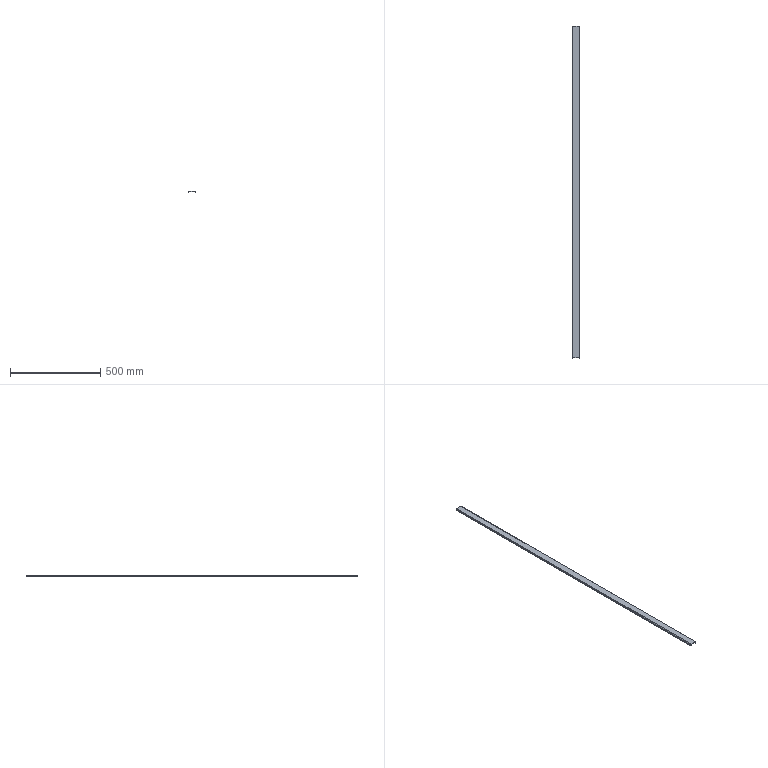Part | SolidWorks | features BaseBody 1 | 1 solid | 22 faces | box 40 x 1838 x 10 mm | volume 245796 mm3 | plane 18 | cylinder 4 | commonest cylinder face diameters 1 x2 6 x2
STEP:
#1=CARTESIAN_POINT('',(-17.5,918.9,-10.));
#2=VERTEX_POINT('',#1);
#3=CARTESIAN_POINT('',(-17.5,-918.9,-10.));
#4=VERTEX_POINT('',#3);
#5=CARTESIAN_POINT('',(-17.5,-918.9,-10.));
#6=DIRECTION('',(0.,-1.,0.));
#7=VECTOR('',#6,1000.);
#8=LINE('',#5,#7);
#9=EDGE_CURVE('',#2,#4,#8,.T.);
#10=ORIENTED_EDGE('',*,*,#9,.T.);
#11=CARTESIAN_POINT('',(-20.,-918.9,-10.));
#12=VERTEX_POINT('',#11);
#13=CARTESIAN_POINT('',(-20.,-918.9,-10.));
#14=DIRECTION('',(1.,0.,0.));
#15=VECTOR('',#14,1000.);
#16=LINE('',#13,#15);
#17=EDGE_CURVE('',#12,#4,#16,.T.);
#18=ORIENTED_EDGE('',*,*,#17,.F.);
#19=CARTESIAN_POINT('',(-20.,918.9,-10.));
#20=VERTEX_POINT('',#19);
#21=CARTESIAN_POINT('',(-20.,0.,-10.));
#22=DIRECTION('',(0.,-1.,0.));
#23=VECTOR('',#22,1000.);
#24=LINE('',#21,#23);
#25=EDGE_CURVE('',#20,#12,#24,.T.);
#26=ORIENTED_EDGE('',*,*,#25,.F.);
#27=CARTESIAN_POINT('',(-20.,918.9,-10.));
#28=DIRECTION('',(1.,0.,0.));
#29=VECTOR('',#28,1000.);
#30=LINE('',#27,#29);
#31=EDGE_CURVE('',#20,#2,#30,.T.);
#32=ORIENTED_EDGE('',*,*,#31,.T.);
#33=EDGE_LOOP('',(#10,#18,#26,#32));
#34=FACE_OUTER_BOUND('',#33,.T.);
#35=CARTESIAN_POINT('',(-20.,-918.9,-10.));
#36=DIRECTION('',(0.,0.,1.));
#37=DIRECTION('',(1.,0.,0.));
#38=AXIS2_PLACEMENT_3D('',#35,#36,#37);
#39=PLANE('',#38);
#40=ADVANCED_FACE('',(#34),#39,.F.);
#41=CARTESIAN_POINT('',(-17.5,918.9,-3.));
#42=VERTEX_POINT('',#41);
#43=CARTESIAN_POINT('',(-17.5,918.9,-10.));
#44=DIRECTION('',(0.,0.,-1.));
#45=VECTOR('',#44,1000.);
#46=LINE('',#43,#45);
#47=EDGE_CURVE('',#42,#2,#46,.T.);
#48=ORIENTED_EDGE('',*,*,#47,.F.);
#49=CARTESIAN_POINT('',(-17.5,-918.9,-3.));
#50=VERTEX_POINT('',#49);
#51=CARTESIAN_POINT('',(-17.5,-918.9,-3.));
#52=DIRECTION('',(0.,1.,0.));
#53=VECTOR('',#52,1000.);
#54=LINE('',#51,#53);
#55=EDGE_CURVE('',#50,#42,#54,.T.);
#56=ORIENTED_EDGE('',*,*,#55,.F.);
#57=CARTESIAN_POINT('',(-17.5,-918.9,-2.5));
#58=DIRECTION('',(0.,0.,1.));
#59=VECTOR('',#58,1000.);
#60=LINE('',#57,#59);
#61=EDGE_CURVE('',#4,#50,#60,.T.);
#62=ORIENTED_EDGE('',*,*,#61,.F.);
#63=ORIENTED_EDGE('',*,*,#9,.F.);
#64=EDGE_LOOP('',(#48,#56,#62,#63));
#65=FACE_OUTER_BOUND('',#64,.T.);
#66=CARTESIAN_POINT('',(-17.5,0.,0.));
#67=DIRECTION('',(1.,0.,0.));
#68=DIRECTION('',(0.,0.,-1.));
#69=AXIS2_PLACEMENT_3D('',#66,#67,#68);
#70=PLANE('',#69);
#71=ADVANCED_FACE('',(#65),#70,.T.);
#72=CARTESIAN_POINT('',(-20.,918.9,-3.));
#73=VERTEX_POINT('',#72);
#74=CARTESIAN_POINT('',(-20.,-918.9,-3.));
#75=VERTEX_POINT('',#74);
#76=CARTESIAN_POINT('',(-20.,-918.9,-3.));
#77=DIRECTION('',(0.,-1.,0.));
#78=VECTOR('',#77,1000.);
#79=LINE('',#76,#78);
#80=EDGE_CURVE('',#73,#75,#79,.T.);
#81=ORIENTED_EDGE('',*,*,#80,.F.);
#82=CARTESIAN_POINT('',(-20.,918.9,0.));
#83=DIRECTION('',(0.,0.,-1.));
#84=VECTOR('',#83,1000.);
#85=LINE('',#82,#84);
#86=EDGE_CURVE('',#73,#20,#85,.T.);
#87=ORIENTED_EDGE('',*,*,#86,.T.);
#88=ORIENTED_EDGE('',*,*,#25,.T.);
#89=CARTESIAN_POINT('',(-20.,-918.9,0.));
#90=DIRECTION('',(0.,0.,1.));
#91=VECTOR('',#90,1000.);
#92=LINE('',#89,#91);
#93=EDGE_CURVE('',#12,#75,#92,.T.);
#94=ORIENTED_EDGE('',*,*,#93,.T.);
#95=EDGE_LOOP('',(#81,#87,#88,#94));
#96=FACE_OUTER_BOUND('',#95,.T.);
#97=CARTESIAN_POINT('',(-20.,0.,0.));
#98=DIRECTION('',(1.,0.,0.));
#99=DIRECTION('',(0.,0.,-1.));
#100=AXIS2_PLACEMENT_3D('',#97,#98,#99);
#101=PLANE('',#100);
#102=ADVANCED_FACE('',(#96),#101,.F.);
#103=CARTESIAN_POINT('',(-20.,-918.9,-3.));
#104=DIRECTION('',(-1.,0.,0.));
#105=VECTOR('',#104,1000.);
#106=LINE('',#103,#105);
#107=EDGE_CURVE('',#50,#75,#106,.T.);
#108=ORIENTED_EDGE('',*,*,#107,.T.);
#109=ORIENTED_EDGE('',*,*,#93,.F.);
#110=ORIENTED_EDGE('',*,*,#17,.T.);
#111=ORIENTED_EDGE('',*,*,#61,.T.);
#112=EDGE_LOOP('',(#108,#109,#110,#111));
#113=FACE_OUTER_BOUND('',#112,.T.);
#114=CARTESIAN_POINT('',(-20.,-918.9,-2.5));
#115=DIRECTION('',(0.,1.,0.));
#116=DIRECTION('',(0.,0.,-1.));
#117=AXIS2_PLACEMENT_3D('',#114,#115,#116);
#118=PLANE('',#117);
#119=ADVANCED_FACE('',(#113),#118,.F.);
#120=CARTESIAN_POINT('',(-17.5,918.9,-3.));
#121=DIRECTION('',(-1.,0.,0.));
#122=VECTOR('',#121,1000.);
#123=LINE('',#120,#122);
#124=EDGE_CURVE('',#42,#73,#123,.T.);
#125=ORIENTED_EDGE('',*,*,#124,.F.);
#126=ORIENTED_EDGE('',*,*,#47,.T.);
#127=ORIENTED_EDGE('',*,*,#31,.F.);
#128=ORIENTED_EDGE('',*,*,#86,.F.);
#129=EDGE_LOOP('',(#125,#126,#127,#128));
#130=FACE_OUTER_BOUND('',#129,.T.);
#131=CARTESIAN_POINT('',(-20.,918.9,-10.));
#132=DIRECTION('',(0.,-1.,0.));
#133=DIRECTION('',(-1.,0.,0.));
#134=AXIS2_PLACEMENT_3D('',#131,#132,#133);
#135=PLANE('',#134);
#136=ADVANCED_FACE('',(#130),#135,.F.);
#137=CARTESIAN_POINT('',(-17.,918.9,-2.5));
#138=VERTEX_POINT('',#137);
#139=CARTESIAN_POINT('',(-17.,-918.9,-2.5));
#140=VERTEX_POINT('',#139);
#141=CARTESIAN_POINT('',(-17.,918.9,-2.5));
#142=DIRECTION('',(0.,-1.,0.));
#143=VECTOR('',#142,1000.);
#144=LINE('',#141,#143);
#145=EDGE_CURVE('',#138,#140,#144,.T.);
#146=ORIENTED_EDGE('',*,*,#145,.T.);
#147=CARTESIAN_POINT('',(-17.,-918.9,-3.));
#148=DIRECTION('',(0.,-1.,0.));
#149=DIRECTION('',(0.,0.,1.));
#150=AXIS2_PLACEMENT_3D('',#147,#148,#149);
#151=CIRCLE('',#150,0.5);
#152=EDGE_CURVE('',#140,#50,#151,.T.);
#153=ORIENTED_EDGE('',*,*,#152,.T.);
#154=ORIENTED_EDGE('',*,*,#55,.T.);
#155=CARTESIAN_POINT('',(-17.,918.9,-3.));
#156=DIRECTION('',(0.,1.,0.));
#157=DIRECTION('',(0.,0.,1.));
#158=AXIS2_PLACEMENT_3D('',#155,#156,#157);
#159=CIRCLE('',#158,0.5);
#160=EDGE_CURVE('',#42,#138,#159,.T.);
#161=ORIENTED_EDGE('',*,*,#160,.T.);
#162=EDGE_LOOP('',(#146,#153,#154,#161));
#163=FACE_OUTER_BOUND('',#162,.T.);
#164=CARTESIAN_POINT('',(-17.,918.9,-3.));
#165=DIRECTION('',(0.,1.,0.));
#166=DIRECTION('',(-1.,0.,0.));
#167=AXIS2_PLACEMENT_3D('',#164,#165,#166);
#168=CYLINDRICAL_SURFACE('',#167,0.5);
#169=ADVANCED_FACE('',(#163),#168,.F.);
#170=CARTESIAN_POINT('',(-17.,918.9,0.));
#171=VERTEX_POINT('',#170);
#172=CARTESIAN_POINT('',(-17.,-918.9,0.));
#173=VERTEX_POINT('',#172);
#174=CARTESIAN_POINT('',(-17.,918.9,0.));
#175=DIRECTION('',(0.,-1.,0.));
#176=VECTOR('',#175,1000.);
#177=LINE('',#174,#176);
#178=EDGE_CURVE('',#171,#173,#177,.T.);
#179=ORIENTED_EDGE('',*,*,#178,.F.);
#180=CARTESIAN_POINT('',(-17.,918.9,-3.));
#181=DIRECTION('',(0.,1.,0.));
#182=DIRECTION('',(0.,0.,1.));
#183=AXIS2_PLACEMENT_3D('',#180,#181,#182);
#184=CIRCLE('',#183,3.);
#185=EDGE_CURVE('',#73,#171,#184,.T.);
#186=ORIENTED_EDGE('',*,*,#185,.F.);
#187=ORIENTED_EDGE('',*,*,#80,.T.);
#188=CARTESIAN_POINT('',(-17.,-918.9,-3.));
#189=DIRECTION('',(0.,-1.,0.));
#190=DIRECTION('',(0.,0.,1.));
#191=AXIS2_PLACEMENT_3D('',#188,#189,#190);
#192=CIRCLE('',#191,3.);
#193=EDGE_CURVE('',#173,#75,#192,.T.);
#194=ORIENTED_EDGE('',*,*,#193,.F.);
#195=EDGE_LOOP('',(#179,#186,#187,#194));
#196=FACE_OUTER_BOUND('',#195,.T.);
#197=CARTESIAN_POINT('',(-17.,918.9,-3.));
#198=DIRECTION('',(0.,1.,0.));
#199=DIRECTION('',(-1.,0.,0.));
#200=AXIS2_PLACEMENT_3D('',#197,#198,#199);
#201=CYLINDRICAL_SURFACE('',#200,3.);
#202=ADVANCED_FACE('',(#196),#201,.T.);
#203=ORIENTED_EDGE('',*,*,#160,.F.);
#204=ORIENTED_EDGE('',*,*,#124,.T.);
#205=ORIENTED_EDGE('',*,*,#185,.T.);
#206=CARTESIAN_POINT('',(-17.,918.9,-2.5));
#207=DIRECTION('',(0.,0.,1.));
#208=VECTOR('',#207,1000.);
#209=LINE('',#206,#208);
#210=EDGE_CURVE('',#138,#171,#209,.T.);
#211=ORIENTED_EDGE('',*,*,#210,.F.);
#212=EDGE_LOOP('',(#203,#204,#205,#211));
#213=FACE_OUTER_BOUND('',#212,.T.);
#214=CARTESIAN_POINT('',(-17.,918.9,-3.));
#215=DIRECTION('',(0.,-1.,0.));
#216=DIRECTION('',(0.,0.,-1.));
#217=AXIS2_PLACEMENT_3D('',#214,#215,#216);
#218=PLANE('',#217);
#219=ADVANCED_FACE('',(#213),#218,.F.);
#220=ORIENTED_EDGE('',*,*,#107,.F.);
#221=ORIENTED_EDGE('',*,*,#152,.F.);
#222=CARTESIAN_POINT('',(-17.,-918.9,-2.5));
#223=DIRECTION('',(0.,0.,1.));
#224=VECTOR('',#223,1000.);
#225=LINE('',#222,#224);
#226=EDGE_CURVE('',#140,#173,#225,.T.);
#227=ORIENTED_EDGE('',*,*,#226,.T.);
#228=ORIENTED_EDGE('',*,*,#193,.T.);
#229=EDGE_LOOP('',(#220,#221,#227,#228));
#230=FACE_OUTER_BOUND('',#229,.T.);
#231=CARTESIAN_POINT('',(-17.,-918.9,-3.));
#232=DIRECTION('',(0.,-1.,0.));
#233=DIRECTION('',(0.,0.,-1.));
#234=AXIS2_PLACEMENT_3D('',#231,#232,#233);
#235=PLANE('',#234);
#236=ADVANCED_FACE('',(#230),#235,.T.);
#237=CARTESIAN_POINT('',(17.5,-918.9,-10.));
#238=VERTEX_POINT('',#237);
#239=CARTESIAN_POINT('',(17.5,918.9,-10.));
#240=VERTEX_POINT('',#239);
#241=CARTESIAN_POINT('',(17.5,918.9,-10.));
#242=DIRECTION('',(0.,1.,0.));
#243=VECTOR('',#242,1000.);
#244=LINE('',#241,#243);
#245=EDGE_CURVE('',#238,#240,#244,.T.);
#246=ORIENTED_EDGE('',*,*,#245,.T.);
#247=CARTESIAN_POINT('',(20.,918.9,-10.));
#248=VERTEX_POINT('',#247);
#249=CARTESIAN_POINT('',(20.,918.9,-10.));
#250=DIRECTION('',(-1.,0.,0.));
#251=VECTOR('',#250,1000.);
#252=LINE('',#249,#251);
#253=EDGE_CURVE('',#248,#240,#252,.T.);
#254=ORIENTED_EDGE('',*,*,#253,.F.);
#255=CARTESIAN_POINT('',(20.,-918.9,-10.));
#256=VERTEX_POINT('',#255);
#257=CARTESIAN_POINT('',(20.,0.,-10.));
#258=DIRECTION('',(0.,1.,0.));
#259=VECTOR('',#258,1000.);
#260=LINE('',#257,#259);
#261=EDGE_CURVE('',#256,#248,#260,.T.);
#262=ORIENTED_EDGE('',*,*,#261,.F.);
#263=CARTESIAN_POINT('',(20.,-918.9,-10.));
#264=DIRECTION('',(-1.,0.,0.));
#265=VECTOR('',#264,1000.);
#266=LINE('',#263,#265);
#267=EDGE_CURVE('',#256,#238,#266,.T.);
#268=ORIENTED_EDGE('',*,*,#267,.T.);
#269=EDGE_LOOP('',(#246,#254,#262,#268));
#270=FACE_OUTER_BOUND('',#269,.T.);
#271=CARTESIAN_POINT('',(20.,918.9,-10.));
#272=DIRECTION('',(0.,0.,1.));
#273=DIRECTION('',(1.,0.,0.));
#274=AXIS2_PLACEMENT_3D('',#271,#272,#273);
#275=PLANE('',#274);
#276=ADVANCED_FACE('',(#270),#275,.F.);
#277=CARTESIAN_POINT('',(17.5,-918.9,-3.));
#278=VERTEX_POINT('',#277);
#279=CARTESIAN_POINT('',(17.5,-918.9,-10.));
#280=DIRECTION('',(0.,0.,-1.));
#281=VECTOR('',#280,1000.);
#282=LINE('',#279,#281);
#283=EDGE_CURVE('',#278,#238,#282,.T.);
#284=ORIENTED_EDGE('',*,*,#283,.F.);
#285=CARTESIAN_POINT('',(17.5,918.9,-3.));
#286=VERTEX_POINT('',#285);
#287=CARTESIAN_POINT('',(17.5,918.9,-3.));
#288=DIRECTION('',(0.,-1.,0.));
#289=VECTOR('',#288,1000.);
#290=LINE('',#287,#289);
#291=EDGE_CURVE('',#286,#278,#290,.T.);
#292=ORIENTED_EDGE('',*,*,#291,.F.);
#293=CARTESIAN_POINT('',(17.5,918.9,-2.5));
#294=DIRECTION('',(0.,0.,1.));
#295=VECTOR('',#294,1000.);
#296=LINE('',#293,#295);
#297=EDGE_CURVE('',#240,#286,#296,.T.);
#298=ORIENTED_EDGE('',*,*,#297,.F.);
#299=ORIENTED_EDGE('',*,*,#245,.F.);
#300=EDGE_LOOP('',(#284,#292,#298,#299));
#301=FACE_OUTER_BOUND('',#300,.T.);
#302=CARTESIAN_POINT('',(17.5,0.,0.));
#303=DIRECTION('',(-1.,0.,0.));
#304=DIRECTION('',(0.,0.,1.));
#305=AXIS2_PLACEMENT_3D('',#302,#303,#304);
#306=PLANE('',#305);
#307=ADVANCED_FACE('',(#301),#306,.T.);
#308=CARTESIAN_POINT('',(20.,-918.9,-3.));
#309=VERTEX_POINT('',#308);
#310=CARTESIAN_POINT('',(20.,918.9,-3.));
#311=VERTEX_POINT('',#310);
#312=CARTESIAN_POINT('',(20.,918.9,-3.));
#313=DIRECTION('',(0.,1.,0.));
#314=VECTOR('',#313,1000.);
#315=LINE('',#312,#314);
#316=EDGE_CURVE('',#309,#311,#315,.T.);
#317=ORIENTED_EDGE('',*,*,#316,.F.);
#318=CARTESIAN_POINT('',(20.,-918.9,0.));
#319=DIRECTION('',(0.,0.,-1.));
#320=VECTOR('',#319,1000.);
#321=LINE('',#318,#320);
#322=EDGE_CURVE('',#309,#256,#321,.T.);
#323=ORIENTED_EDGE('',*,*,#322,.T.);
#324=ORIENTED_EDGE('',*,*,#261,.T.);
#325=CARTESIAN_POINT('',(20.,918.9,0.));
#326=DIRECTION('',(0.,0.,1.));
#327=VECTOR('',#326,1000.);
#328=LINE('',#325,#327);
#329=EDGE_CURVE('',#248,#311,#328,.T.);
#330=ORIENTED_EDGE('',*,*,#329,.T.);
#331=EDGE_LOOP('',(#317,#323,#324,#330));
#332=FACE_OUTER_BOUND('',#331,.T.);
#333=CARTESIAN_POINT('',(20.,0.,0.));
#334=DIRECTION('',(-1.,0.,0.));
#335=DIRECTION('',(0.,0.,1.));
#336=AXIS2_PLACEMENT_3D('',#333,#334,#335);
#337=PLANE('',#336);
#338=ADVANCED_FACE('',(#332),#337,.F.);
#339=CARTESIAN_POINT('',(20.,918.9,-3.));
#340=DIRECTION('',(1.,0.,0.));
#341=VECTOR('',#340,1000.);
#342=LINE('',#339,#341);
#343=EDGE_CURVE('',#286,#311,#342,.T.);
#344=ORIENTED_EDGE('',*,*,#343,.T.);
#345=ORIENTED_EDGE('',*,*,#329,.F.);
#346=ORIENTED_EDGE('',*,*,#253,.T.);
#347=ORIENTED_EDGE('',*,*,#297,.T.);
#348=EDGE_LOOP('',(#344,#345,#346,#347));
#349=FACE_OUTER_BOUND('',#348,.T.);
#350=CARTESIAN_POINT('',(20.,918.9,-2.5));
#351=DIRECTION('',(0.,-1.,0.));
#352=DIRECTION('',(-1.,0.,0.));
#353=AXIS2_PLACEMENT_3D('',#350,#351,#352);
#354=PLANE('',#353);
#355=ADVANCED_FACE('',(#349),#354,.F.);
#356=CARTESIAN_POINT('',(17.5,-918.9,-3.));
#357=DIRECTION('',(1.,0.,0.));
#358=VECTOR('',#357,1000.);
#359=LINE('',#356,#358);
#360=EDGE_CURVE('',#278,#309,#359,.T.);
#361=ORIENTED_EDGE('',*,*,#360,.F.);
#362=ORIENTED_EDGE('',*,*,#283,.T.);
#363=ORIENTED_EDGE('',*,*,#267,.F.);
#364=ORIENTED_EDGE('',*,*,#322,.F.);
#365=EDGE_LOOP('',(#361,#362,#363,#364));
#366=FACE_OUTER_BOUND('',#365,.T.);
#367=CARTESIAN_POINT('',(20.,-918.9,-10.));
#368=DIRECTION('',(0.,1.,0.));
#369=DIRECTION('',(0.,0.,-1.));
#370=AXIS2_PLACEMENT_3D('',#367,#368,#369);
#371=PLANE('',#370);
#372=ADVANCED_FACE('',(#366),#371,.F.);
#373=CARTESIAN_POINT('',(17.,-918.9,-2.5));
#374=VERTEX_POINT('',#373);
#375=CARTESIAN_POINT('',(17.,918.9,-2.5));
#376=VERTEX_POINT('',#375);
#377=CARTESIAN_POINT('',(17.,-918.9,-2.5));
#378=DIRECTION('',(0.,1.,0.));
#379=VECTOR('',#378,1000.);
#380=LINE('',#377,#379);
#381=EDGE_CURVE('',#374,#376,#380,.T.);
#382=ORIENTED_EDGE('',*,*,#381,.T.);
#383=CARTESIAN_POINT('',(17.,918.9,-3.));
#384=DIRECTION('',(0.,1.,0.));
#385=DIRECTION('',(0.,0.,-1.));
#386=AXIS2_PLACEMENT_3D('',#383,#384,#385);
#387=CIRCLE('',#386,0.5);
#388=EDGE_CURVE('',#376,#286,#387,.T.);
#389=ORIENTED_EDGE('',*,*,#388,.T.);
#390=ORIENTED_EDGE('',*,*,#291,.T.);
#391=CARTESIAN_POINT('',(17.,-918.9,-3.));
#392=DIRECTION('',(0.,-1.,0.));
#393=DIRECTION('',(0.,0.,-1.));
#394=AXIS2_PLACEMENT_3D('',#391,#392,#393);
#395=CIRCLE('',#394,0.5);
#396=EDGE_CURVE('',#278,#374,#395,.T.);
#397=ORIENTED_EDGE('',*,*,#396,.T.);
#398=EDGE_LOOP('',(#382,#389,#390,#397));
#399=FACE_OUTER_BOUND('',#398,.T.);
#400=CARTESIAN_POINT('',(17.,-918.9,-3.));
#401=DIRECTION('',(0.,-1.,0.));
#402=DIRECTION('',(1.,0.,0.));
#403=AXIS2_PLACEMENT_3D('',#400,#401,#402);
#404=CYLINDRICAL_SURFACE('',#403,0.5);
#405=ADVANCED_FACE('',(#399),#404,.F.);
#406=CARTESIAN_POINT('',(17.,-918.9,0.));
#407=VERTEX_POINT('',#406);
#408=CARTESIAN_POINT('',(17.,918.9,0.));
#409=VERTEX_POINT('',#408);
#410=CARTESIAN_POINT('',(17.,-918.9,0.));
#411=DIRECTION('',(0.,1.,0.));
#412=VECTOR('',#411,1000.);
#413=LINE('',#410,#412);
#414=EDGE_CURVE('',#407,#409,#413,.T.);
#415=ORIENTED_EDGE('',*,*,#414,.F.);
#416=CARTESIAN_POINT('',(17.,-918.9,-3.));
#417=DIRECTION('',(0.,-1.,0.));
#418=DIRECTION('',(0.,0.,-1.));
#419=AXIS2_PLACEMENT_3D('',#416,#417,#418);
#420=CIRCLE('',#419,3.);
#421=EDGE_CURVE('',#309,#407,#420,.T.);
#422=ORIENTED_EDGE('',*,*,#421,.F.);
#423=ORIENTED_EDGE('',*,*,#316,.T.);
#424=CARTESIAN_POINT('',(17.,918.9,-3.));
#425=DIRECTION('',(0.,1.,0.));
#426=DIRECTION('',(0.,0.,-1.));
#427=AXIS2_PLACEMENT_3D('',#424,#425,#426);
#428=CIRCLE('',#427,3.);
#429=EDGE_CURVE('',#409,#311,#428,.T.);
#430=ORIENTED_EDGE('',*,*,#429,.F.);
#431=EDGE_LOOP('',(#415,#422,#423,#430));
#432=FACE_OUTER_BOUND('',#431,.T.);
#433=CARTESIAN_POINT('',(17.,-918.9,-3.));
#434=DIRECTION('',(0.,-1.,0.));
#435=DIRECTION('',(1.,0.,0.));
#436=AXIS2_PLACEMENT_3D('',#433,#434,#435);
#437=CYLINDRICAL_SURFACE('',#436,3.);
#438=ADVANCED_FACE('',(#432),#437,.T.);
#439=ORIENTED_EDGE('',*,*,#396,.F.);
#440=ORIENTED_EDGE('',*,*,#360,.T.);
#441=ORIENTED_EDGE('',*,*,#421,.T.);
#442=CARTESIAN_POINT('',(17.,-918.9,-2.5));
#443=DIRECTION('',(0.,0.,1.));
#444=VECTOR('',#443,1000.);
#445=LINE('',#442,#444);
#446=EDGE_CURVE('',#374,#407,#445,.T.);
#447=ORIENTED_EDGE('',*,*,#446,.F.);
#448=EDGE_LOOP('',(#439,#440,#441,#447));
#449=FACE_OUTER_BOUND('',#448,.T.);
#450=CARTESIAN_POINT('',(17.,-918.9,-3.));
#451=DIRECTION('',(0.,1.,0.));
#452=DIRECTION('',(1.,0.,0.));
#453=AXIS2_PLACEMENT_3D('',#450,#451,#452);
#454=PLANE('',#453);
#455=ADVANCED_FACE('',(#449),#454,.F.);
#456=ORIENTED_EDGE('',*,*,#343,.F.);
#457=ORIENTED_EDGE('',*,*,#388,.F.);
#458=CARTESIAN_POINT('',(17.,918.9,-2.5));
#459=DIRECTION('',(0.,0.,1.));
#460=VECTOR('',#459,1000.);
#461=LINE('',#458,#460);
#462=EDGE_CURVE('',#376,#409,#461,.T.);
#463=ORIENTED_EDGE('',*,*,#462,.T.);
#464=ORIENTED_EDGE('',*,*,#429,.T.);
#465=EDGE_LOOP('',(#456,#457,#463,#464));
#466=FACE_OUTER_BOUND('',#465,.T.);
#467=CARTESIAN_POINT('',(17.,918.9,-3.));
#468=DIRECTION('',(0.,1.,0.));
#469=DIRECTION('',(1.,0.,0.));
#470=AXIS2_PLACEMENT_3D('',#467,#468,#469);
#471=PLANE('',#470);
#472=ADVANCED_FACE('',(#466),#471,.T.);
#473=ORIENTED_EDGE('',*,*,#226,.F.);
#474=CARTESIAN_POINT('',(20.,-918.9,-2.5));
#475=DIRECTION('',(1.,0.,0.));
#476=VECTOR('',#475,1000.);
#477=LINE('',#474,#476);
#478=EDGE_CURVE('',#140,#374,#477,.T.);
#479=ORIENTED_EDGE('',*,*,#478,.T.);
#480=ORIENTED_EDGE('',*,*,#446,.T.);
#481=CARTESIAN_POINT('',(20.,-918.9,0.));
#482=DIRECTION('',(1.,0.,0.));
#483=VECTOR('',#482,1000.);
#484=LINE('',#481,#483);
#485=EDGE_CURVE('',#173,#407,#484,.T.);
#486=ORIENTED_EDGE('',*,*,#485,.F.);
#487=EDGE_LOOP('',(#473,#479,#480,#486));
#488=FACE_OUTER_BOUND('',#487,.T.);
#489=CARTESIAN_POINT('',(20.,-918.9,-2.5));
#490=DIRECTION('',(0.,-1.,0.));
#491=DIRECTION('',(0.,0.,-1.));
#492=AXIS2_PLACEMENT_3D('',#489,#490,#491);
#493=PLANE('',#492);
#494=ADVANCED_FACE('',(#488),#493,.T.);
#495=CARTESIAN_POINT('',(20.,918.9,-2.5));
#496=DIRECTION('',(-1.,0.,0.));
#497=VECTOR('',#496,1000.);
#498=LINE('',#495,#497);
#499=EDGE_CURVE('',#376,#138,#498,.T.);
#500=ORIENTED_EDGE('',*,*,#499,.T.);
#501=ORIENTED_EDGE('',*,*,#210,.T.);
#502=CARTESIAN_POINT('',(20.,918.9,0.));
#503=DIRECTION('',(-1.,0.,0.));
#504=VECTOR('',#503,1000.);
#505=LINE('',#502,#504);
#506=EDGE_CURVE('',#409,#171,#505,.T.);
#507=ORIENTED_EDGE('',*,*,#506,.F.);
#508=ORIENTED_EDGE('',*,*,#462,.F.);
#509=EDGE_LOOP('',(#500,#501,#507,#508));
#510=FACE_OUTER_BOUND('',#509,.T.);
#511=CARTESIAN_POINT('',(20.,918.9,-2.5));
#512=DIRECTION('',(0.,1.,0.));
#513=DIRECTION('',(1.,0.,0.));
#514=AXIS2_PLACEMENT_3D('',#511,#512,#513);
#515=PLANE('',#514);
#516=ADVANCED_FACE('',(#510),#515,.T.);
#517=ORIENTED_EDGE('',*,*,#178,.T.);
#518=ORIENTED_EDGE('',*,*,#485,.T.);
#519=ORIENTED_EDGE('',*,*,#414,.T.);
#520=ORIENTED_EDGE('',*,*,#506,.T.);
#521=EDGE_LOOP('',(#517,#518,#519,#520));
#522=FACE_OUTER_BOUND('',#521,.T.);
#523=CARTESIAN_POINT('',(0.,0.,0.));
#524=DIRECTION('',(0.,0.,-1.));
#525=DIRECTION('',(0.,-1.,0.));
#526=AXIS2_PLACEMENT_3D('',#523,#524,#525);
#527=PLANE('',#526);
#528=ADVANCED_FACE('',(#522),#527,.F.);
#529=ORIENTED_EDGE('',*,*,#478,.F.);
#530=ORIENTED_EDGE('',*,*,#145,.F.);
#531=ORIENTED_EDGE('',*,*,#499,.F.);
#532=ORIENTED_EDGE('',*,*,#381,.F.);
#533=EDGE_LOOP('',(#529,#530,#531,#532));
#534=FACE_OUTER_BOUND('',#533,.T.);
#535=CARTESIAN_POINT('',(0.,0.,-2.5));
#536=DIRECTION('',(0.,0.,-1.));
#537=DIRECTION('',(0.,-1.,0.));
#538=AXIS2_PLACEMENT_3D('',#535,#536,#537);
#539=PLANE('',#538);
#540=ADVANCED_FACE('',(#534),#539,.T.);
#541=CLOSED_SHELL('',(#40,#71,#102,#119,#136,#169,#202,#219,#236,#276,#307,#338,#355,#372,#405,#438,#455,#472,#494,#516,#528,#540));
#542=MANIFOLD_SOLID_BREP('',#541);
#543=CARTESIAN_POINT('',(0.,0.,0.));
#544=DIRECTION('',(0.,0.,1.));
#545=DIRECTION('',(1.,0.,0.));
#546=AXIS2_PLACEMENT_3D('',#543,#544,#545);
#547=(LENGTH_UNIT()NAMED_UNIT(*)SI_UNIT(.MILLI.,.METRE.));
#548=UNCERTAINTY_MEASURE_WITH_UNIT(LENGTH_MEASURE(0.00001),#547,'','');
#549=(NAMED_UNIT(*)PLANE_ANGLE_UNIT()SI_UNIT($,.RADIAN.));
#550=(NAMED_UNIT(*)SI_UNIT($,.STERADIAN.)SOLID_ANGLE_UNIT());
#551=(GEOMETRIC_REPRESENTATION_CONTEXT(3)GLOBAL_UNCERTAINTY_ASSIGNED_CONTEXT((#548))GLOBAL_UNIT_ASSIGNED_CONTEXT((#547,#549,#550))REPRESENTATION_CONTEXT('',''));
#552=ADVANCED_BREP_SHAPE_REPRESENTATION('',(#542,#546),#551);